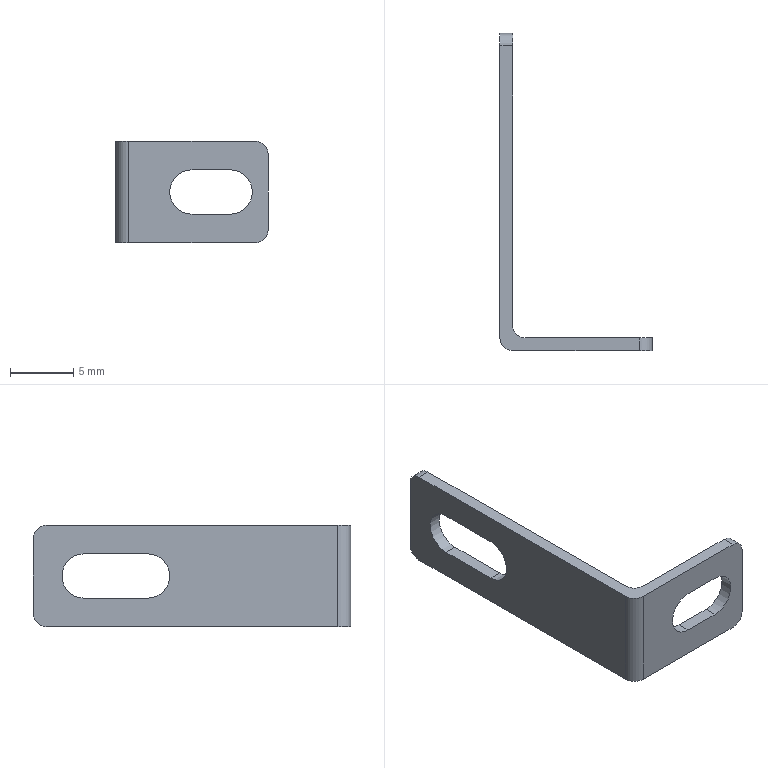Part | SolidWorks | features ICE 2, ExtruThin 1, Fillet 1 | 1 solid | 22 faces | box 12 x 25 x 8 mm | volume 239.899 mm3 | plane 12 | cylinder 10 | commonest cylinder face diameters 2 x6 3.5 x4
STEP:
#1=CARTESIAN_POINT('',(9.,0.,-1.75));
#2=VERTEX_POINT('',#1);
#3=CARTESIAN_POINT('',(6.,0.,-1.75));
#4=VERTEX_POINT('',#3);
#5=CARTESIAN_POINT('',(6.,0.,-1.75));
#6=DIRECTION('',(-1.,0.,0.));
#7=VECTOR('',#6,1000.);
#8=LINE('',#5,#7);
#9=EDGE_CURVE('',#2,#4,#8,.T.);
#10=ORIENTED_EDGE('',*,*,#9,.T.);
#11=CARTESIAN_POINT('',(6.,0.,1.75));
#12=VERTEX_POINT('',#11);
#13=CARTESIAN_POINT('',(6.,0.,0.));
#14=DIRECTION('',(0.,1.,0.));
#15=DIRECTION('',(0.,0.,1.));
#16=AXIS2_PLACEMENT_3D('',#13,#14,#15);
#17=CIRCLE('',#16,1.75);
#18=EDGE_CURVE('',#4,#12,#17,.T.);
#19=ORIENTED_EDGE('',*,*,#18,.T.);
#20=CARTESIAN_POINT('',(9.,0.,1.75));
#21=VERTEX_POINT('',#20);
#22=CARTESIAN_POINT('',(6.,0.,1.75));
#23=DIRECTION('',(1.,0.,0.));
#24=VECTOR('',#23,1000.);
#25=LINE('',#22,#24);
#26=EDGE_CURVE('',#12,#21,#25,.T.);
#27=ORIENTED_EDGE('',*,*,#26,.T.);
#28=CARTESIAN_POINT('',(9.,0.,0.));
#29=DIRECTION('',(0.,1.,0.));
#30=DIRECTION('',(0.,0.,1.));
#31=AXIS2_PLACEMENT_3D('',#28,#29,#30);
#32=CIRCLE('',#31,1.75);
#33=EDGE_CURVE('',#21,#2,#32,.T.);
#34=ORIENTED_EDGE('',*,*,#33,.T.);
#35=EDGE_LOOP('',(#10,#19,#27,#34));
#36=FACE_BOUND('',#35,.T.);
#37=CARTESIAN_POINT('',(1.,0.,-4.));
#38=VERTEX_POINT('',#37);
#39=CARTESIAN_POINT('',(11.,0.,-4.));
#40=VERTEX_POINT('',#39);
#41=CARTESIAN_POINT('',(0.,0.,-4.));
#42=DIRECTION('',(1.,0.,0.));
#43=VECTOR('',#42,1000.);
#44=LINE('',#41,#43);
#45=EDGE_CURVE('',#38,#40,#44,.T.);
#46=ORIENTED_EDGE('',*,*,#45,.T.);
#47=CARTESIAN_POINT('',(12.,0.,-3.));
#48=VERTEX_POINT('',#47);
#49=CARTESIAN_POINT('',(11.,0.,-3.));
#50=DIRECTION('',(0.,-1.,0.));
#51=DIRECTION('',(0.,0.,1.));
#52=AXIS2_PLACEMENT_3D('',#49,#50,#51);
#53=CIRCLE('',#52,1.);
#54=EDGE_CURVE('',#40,#48,#53,.T.);
#55=ORIENTED_EDGE('',*,*,#54,.T.);
#56=CARTESIAN_POINT('',(12.,0.,3.));
#57=VERTEX_POINT('',#56);
#58=CARTESIAN_POINT('',(12.,0.,4.));
#59=DIRECTION('',(0.,0.,-1.));
#60=VECTOR('',#59,1000.);
#61=LINE('',#58,#60);
#62=EDGE_CURVE('',#57,#48,#61,.T.);
#63=ORIENTED_EDGE('',*,*,#62,.F.);
#64=CARTESIAN_POINT('',(11.,0.,4.));
#65=VERTEX_POINT('',#64);
#66=CARTESIAN_POINT('',(11.,0.,3.));
#67=DIRECTION('',(0.,-1.,0.));
#68=DIRECTION('',(0.,0.,1.));
#69=AXIS2_PLACEMENT_3D('',#66,#67,#68);
#70=CIRCLE('',#69,1.);
#71=EDGE_CURVE('',#57,#65,#70,.T.);
#72=ORIENTED_EDGE('',*,*,#71,.T.);
#73=CARTESIAN_POINT('',(1.,0.,4.));
#74=VERTEX_POINT('',#73);
#75=CARTESIAN_POINT('',(0.,0.,4.));
#76=DIRECTION('',(1.,0.,0.));
#77=VECTOR('',#76,1000.);
#78=LINE('',#75,#77);
#79=EDGE_CURVE('',#74,#65,#78,.T.);
#80=ORIENTED_EDGE('',*,*,#79,.F.);
#81=CARTESIAN_POINT('',(1.,0.,4.));
#82=DIRECTION('',(0.,0.,-1.));
#83=VECTOR('',#82,1000.);
#84=LINE('',#81,#83);
#85=EDGE_CURVE('',#74,#38,#84,.T.);
#86=ORIENTED_EDGE('',*,*,#85,.T.);
#87=EDGE_LOOP('',(#46,#55,#63,#72,#80,#86));
#88=FACE_OUTER_BOUND('',#87,.T.);
#89=CARTESIAN_POINT('',(0.,0.,4.));
#90=DIRECTION('',(0.,1.,0.));
#91=DIRECTION('',(0.,0.,1.));
#92=AXIS2_PLACEMENT_3D('',#89,#90,#91);
#93=PLANE('',#92);
#94=ADVANCED_FACE('',(#36,#88),#93,.F.);
#95=ORIENTED_EDGE('',*,*,#62,.T.);
#96=CARTESIAN_POINT('',(12.,1.,-3.));
#97=VERTEX_POINT('',#96);
#98=CARTESIAN_POINT('',(12.,1.,-3.));
#99=DIRECTION('',(0.,1.,0.));
#100=VECTOR('',#99,1000.);
#101=LINE('',#98,#100);
#102=EDGE_CURVE('',#48,#97,#101,.T.);
#103=ORIENTED_EDGE('',*,*,#102,.T.);
#104=CARTESIAN_POINT('',(12.,1.,3.));
#105=VERTEX_POINT('',#104);
#106=CARTESIAN_POINT('',(12.,1.,4.));
#107=DIRECTION('',(0.,0.,-1.));
#108=VECTOR('',#107,1000.);
#109=LINE('',#106,#108);
#110=EDGE_CURVE('',#105,#97,#109,.T.);
#111=ORIENTED_EDGE('',*,*,#110,.F.);
#112=CARTESIAN_POINT('',(12.,0.,3.));
#113=DIRECTION('',(0.,-1.,0.));
#114=VECTOR('',#113,1000.);
#115=LINE('',#112,#114);
#116=EDGE_CURVE('',#105,#57,#115,.T.);
#117=ORIENTED_EDGE('',*,*,#116,.T.);
#118=EDGE_LOOP('',(#95,#103,#111,#117));
#119=FACE_OUTER_BOUND('',#118,.T.);
#120=CARTESIAN_POINT('',(12.,1.,4.));
#121=DIRECTION('',(1.,0.,0.));
#122=DIRECTION('',(0.,0.,-1.));
#123=AXIS2_PLACEMENT_3D('',#120,#121,#122);
#124=PLANE('',#123);
#125=ADVANCED_FACE('',(#119),#124,.T.);
#126=CARTESIAN_POINT('',(6.,1.,-1.75));
#127=VERTEX_POINT('',#126);
#128=CARTESIAN_POINT('',(6.,1.,1.75));
#129=VERTEX_POINT('',#128);
#130=CARTESIAN_POINT('',(6.,1.,0.));
#131=DIRECTION('',(0.,1.,0.));
#132=DIRECTION('',(0.,0.,1.));
#133=AXIS2_PLACEMENT_3D('',#130,#131,#132);
#134=CIRCLE('',#133,1.75);
#135=EDGE_CURVE('',#127,#129,#134,.T.);
#136=ORIENTED_EDGE('',*,*,#135,.F.);
#137=CARTESIAN_POINT('',(9.,1.,-1.75));
#138=VERTEX_POINT('',#137);
#139=CARTESIAN_POINT('',(6.,1.,-1.75));
#140=DIRECTION('',(-1.,0.,0.));
#141=VECTOR('',#140,1000.);
#142=LINE('',#139,#141);
#143=EDGE_CURVE('',#138,#127,#142,.T.);
#144=ORIENTED_EDGE('',*,*,#143,.F.);
#145=CARTESIAN_POINT('',(9.,1.,1.75));
#146=VERTEX_POINT('',#145);
#147=CARTESIAN_POINT('',(9.,1.,0.));
#148=DIRECTION('',(0.,1.,0.));
#149=DIRECTION('',(0.,0.,1.));
#150=AXIS2_PLACEMENT_3D('',#147,#148,#149);
#151=CIRCLE('',#150,1.75);
#152=EDGE_CURVE('',#146,#138,#151,.T.);
#153=ORIENTED_EDGE('',*,*,#152,.F.);
#154=CARTESIAN_POINT('',(6.,1.,1.75));
#155=DIRECTION('',(1.,0.,0.));
#156=VECTOR('',#155,1000.);
#157=LINE('',#154,#156);
#158=EDGE_CURVE('',#129,#146,#157,.T.);
#159=ORIENTED_EDGE('',*,*,#158,.F.);
#160=EDGE_LOOP('',(#136,#144,#153,#159));
#161=FACE_BOUND('',#160,.T.);
#162=ORIENTED_EDGE('',*,*,#110,.T.);
#163=CARTESIAN_POINT('',(11.,1.,-4.));
#164=VERTEX_POINT('',#163);
#165=CARTESIAN_POINT('',(11.,1.,-3.));
#166=DIRECTION('',(0.,1.,0.));
#167=DIRECTION('',(0.,0.,1.));
#168=AXIS2_PLACEMENT_3D('',#165,#166,#167);
#169=CIRCLE('',#168,1.);
#170=EDGE_CURVE('',#97,#164,#169,.T.);
#171=ORIENTED_EDGE('',*,*,#170,.T.);
#172=CARTESIAN_POINT('',(2.,1.,-4.));
#173=VERTEX_POINT('',#172);
#174=CARTESIAN_POINT('',(0.,1.,-4.));
#175=DIRECTION('',(1.,0.,0.));
#176=VECTOR('',#175,1000.);
#177=LINE('',#174,#176);
#178=EDGE_CURVE('',#173,#164,#177,.T.);
#179=ORIENTED_EDGE('',*,*,#178,.F.);
#180=CARTESIAN_POINT('',(2.,1.,4.));
#181=VERTEX_POINT('',#180);
#182=CARTESIAN_POINT('',(2.,1.,4.));
#183=DIRECTION('',(0.,0.,1.));
#184=VECTOR('',#183,1000.);
#185=LINE('',#182,#184);
#186=EDGE_CURVE('',#173,#181,#185,.T.);
#187=ORIENTED_EDGE('',*,*,#186,.T.);
#188=CARTESIAN_POINT('',(11.,1.,4.));
#189=VERTEX_POINT('',#188);
#190=CARTESIAN_POINT('',(0.,1.,4.));
#191=DIRECTION('',(1.,0.,0.));
#192=VECTOR('',#191,1000.);
#193=LINE('',#190,#192);
#194=EDGE_CURVE('',#181,#189,#193,.T.);
#195=ORIENTED_EDGE('',*,*,#194,.T.);
#196=CARTESIAN_POINT('',(11.,1.,3.));
#197=DIRECTION('',(0.,1.,0.));
#198=DIRECTION('',(0.,0.,1.));
#199=AXIS2_PLACEMENT_3D('',#196,#197,#198);
#200=CIRCLE('',#199,1.);
#201=EDGE_CURVE('',#189,#105,#200,.T.);
#202=ORIENTED_EDGE('',*,*,#201,.T.);
#203=EDGE_LOOP('',(#162,#171,#179,#187,#195,#202));
#204=FACE_OUTER_BOUND('',#203,.T.);
#205=CARTESIAN_POINT('',(0.,1.,4.));
#206=DIRECTION('',(0.,1.,0.));
#207=DIRECTION('',(0.,0.,1.));
#208=AXIS2_PLACEMENT_3D('',#205,#206,#207);
#209=PLANE('',#208);
#210=ADVANCED_FACE('',(#161,#204),#209,.T.);
#211=CARTESIAN_POINT('',(1.,16.,1.75));
#212=VERTEX_POINT('',#211);
#213=CARTESIAN_POINT('',(1.,16.,-1.75));
#214=VERTEX_POINT('',#213);
#215=CARTESIAN_POINT('',(1.,16.,0.));
#216=DIRECTION('',(1.,0.,0.));
#217=DIRECTION('',(0.,0.,-1.));
#218=AXIS2_PLACEMENT_3D('',#215,#216,#217);
#219=CIRCLE('',#218,1.75);
#220=EDGE_CURVE('',#212,#214,#219,.T.);
#221=ORIENTED_EDGE('',*,*,#220,.F.);
#222=CARTESIAN_POINT('',(1.,21.,1.75));
#223=VERTEX_POINT('',#222);
#224=CARTESIAN_POINT('',(1.,0.,1.75));
#225=DIRECTION('',(0.,-1.,0.));
#226=VECTOR('',#225,1000.);
#227=LINE('',#224,#226);
#228=EDGE_CURVE('',#223,#212,#227,.T.);
#229=ORIENTED_EDGE('',*,*,#228,.F.);
#230=CARTESIAN_POINT('',(1.,21.,-1.75));
#231=VERTEX_POINT('',#230);
#232=CARTESIAN_POINT('',(1.,21.,0.));
#233=DIRECTION('',(1.,0.,0.));
#234=DIRECTION('',(0.,0.,-1.));
#235=AXIS2_PLACEMENT_3D('',#232,#233,#234);
#236=CIRCLE('',#235,1.75);
#237=EDGE_CURVE('',#231,#223,#236,.T.);
#238=ORIENTED_EDGE('',*,*,#237,.F.);
#239=CARTESIAN_POINT('',(1.,0.,-1.75));
#240=DIRECTION('',(0.,1.,0.));
#241=VECTOR('',#240,1000.);
#242=LINE('',#239,#241);
#243=EDGE_CURVE('',#214,#231,#242,.T.);
#244=ORIENTED_EDGE('',*,*,#243,.F.);
#245=EDGE_LOOP('',(#221,#229,#238,#244));
#246=FACE_BOUND('',#245,.T.);
#247=CARTESIAN_POINT('',(1.,24.,-4.));
#248=VERTEX_POINT('',#247);
#249=CARTESIAN_POINT('',(1.,2.,-4.));
#250=VERTEX_POINT('',#249);
#251=CARTESIAN_POINT('',(1.,0.,-4.));
#252=DIRECTION('',(0.,-1.,0.));
#253=VECTOR('',#252,1000.);
#254=LINE('',#251,#253);
#255=EDGE_CURVE('',#248,#250,#254,.T.);
#256=ORIENTED_EDGE('',*,*,#255,.F.);
#257=CARTESIAN_POINT('',(1.,25.,-3.));
#258=VERTEX_POINT('',#257);
#259=CARTESIAN_POINT('',(1.,24.,-3.));
#260=DIRECTION('',(1.,0.,0.));
#261=DIRECTION('',(0.,0.,-1.));
#262=AXIS2_PLACEMENT_3D('',#259,#260,#261);
#263=CIRCLE('',#262,1.);
#264=EDGE_CURVE('',#248,#258,#263,.T.);
#265=ORIENTED_EDGE('',*,*,#264,.T.);
#266=CARTESIAN_POINT('',(1.,25.,3.));
#267=VERTEX_POINT('',#266);
#268=CARTESIAN_POINT('',(1.,25.,4.));
#269=DIRECTION('',(0.,0.,-1.));
#270=VECTOR('',#269,1000.);
#271=LINE('',#268,#270);
#272=EDGE_CURVE('',#267,#258,#271,.T.);
#273=ORIENTED_EDGE('',*,*,#272,.F.);
#274=CARTESIAN_POINT('',(1.,24.,4.));
#275=VERTEX_POINT('',#274);
#276=CARTESIAN_POINT('',(1.,24.,3.));
#277=DIRECTION('',(1.,0.,0.));
#278=DIRECTION('',(0.,0.,-1.));
#279=AXIS2_PLACEMENT_3D('',#276,#277,#278);
#280=CIRCLE('',#279,1.);
#281=EDGE_CURVE('',#267,#275,#280,.T.);
#282=ORIENTED_EDGE('',*,*,#281,.T.);
#283=CARTESIAN_POINT('',(1.,2.,4.));
#284=VERTEX_POINT('',#283);
#285=CARTESIAN_POINT('',(1.,0.,4.));
#286=DIRECTION('',(0.,-1.,0.));
#287=VECTOR('',#286,1000.);
#288=LINE('',#285,#287);
#289=EDGE_CURVE('',#275,#284,#288,.T.);
#290=ORIENTED_EDGE('',*,*,#289,.T.);
#291=CARTESIAN_POINT('',(1.,2.,-4.));
#292=DIRECTION('',(0.,0.,-1.));
#293=VECTOR('',#292,1000.);
#294=LINE('',#291,#293);
#295=EDGE_CURVE('',#284,#250,#294,.T.);
#296=ORIENTED_EDGE('',*,*,#295,.T.);
#297=EDGE_LOOP('',(#256,#265,#273,#282,#290,#296));
#298=FACE_OUTER_BOUND('',#297,.T.);
#299=CARTESIAN_POINT('',(1.,0.,4.));
#300=DIRECTION('',(1.,0.,0.));
#301=DIRECTION('',(0.,0.,-1.));
#302=AXIS2_PLACEMENT_3D('',#299,#300,#301);
#303=PLANE('',#302);
#304=ADVANCED_FACE('',(#246,#298),#303,.T.);
#305=ORIENTED_EDGE('',*,*,#272,.T.);
#306=CARTESIAN_POINT('',(0.,25.,-3.));
#307=VERTEX_POINT('',#306);
#308=CARTESIAN_POINT('',(0.,25.,-3.));
#309=DIRECTION('',(-1.,0.,0.));
#310=VECTOR('',#309,1000.);
#311=LINE('',#308,#310);
#312=EDGE_CURVE('',#258,#307,#311,.T.);
#313=ORIENTED_EDGE('',*,*,#312,.T.);
#314=CARTESIAN_POINT('',(0.,25.,3.));
#315=VERTEX_POINT('',#314);
#316=CARTESIAN_POINT('',(0.,25.,4.));
#317=DIRECTION('',(0.,0.,-1.));
#318=VECTOR('',#317,1000.);
#319=LINE('',#316,#318);
#320=EDGE_CURVE('',#315,#307,#319,.T.);
#321=ORIENTED_EDGE('',*,*,#320,.F.);
#322=CARTESIAN_POINT('',(1.,25.,3.));
#323=DIRECTION('',(1.,0.,0.));
#324=VECTOR('',#323,1000.);
#325=LINE('',#322,#324);
#326=EDGE_CURVE('',#315,#267,#325,.T.);
#327=ORIENTED_EDGE('',*,*,#326,.T.);
#328=EDGE_LOOP('',(#305,#313,#321,#327));
#329=FACE_OUTER_BOUND('',#328,.T.);
#330=CARTESIAN_POINT('',(0.,25.,4.));
#331=DIRECTION('',(0.,1.,0.));
#332=DIRECTION('',(0.,0.,1.));
#333=AXIS2_PLACEMENT_3D('',#330,#331,#332);
#334=PLANE('',#333);
#335=ADVANCED_FACE('',(#329),#334,.T.);
#336=CARTESIAN_POINT('',(0.,16.,1.75));
#337=VERTEX_POINT('',#336);
#338=CARTESIAN_POINT('',(0.,21.,1.75));
#339=VERTEX_POINT('',#338);
#340=CARTESIAN_POINT('',(0.,16.,1.75));
#341=DIRECTION('',(0.,1.,0.));
#342=VECTOR('',#341,1000.);
#343=LINE('',#340,#342);
#344=EDGE_CURVE('',#337,#339,#343,.T.);
#345=ORIENTED_EDGE('',*,*,#344,.F.);
#346=CARTESIAN_POINT('',(0.,16.,-1.75));
#347=VERTEX_POINT('',#346);
#348=CARTESIAN_POINT('',(0.,16.,0.));
#349=DIRECTION('',(-1.,0.,0.));
#350=DIRECTION('',(0.,0.,1.));
#351=AXIS2_PLACEMENT_3D('',#348,#349,#350);
#352=CIRCLE('',#351,1.75);
#353=EDGE_CURVE('',#347,#337,#352,.T.);
#354=ORIENTED_EDGE('',*,*,#353,.F.);
#355=CARTESIAN_POINT('',(0.,21.,-1.75));
#356=VERTEX_POINT('',#355);
#357=CARTESIAN_POINT('',(0.,16.,-1.75));
#358=DIRECTION('',(0.,-1.,0.));
#359=VECTOR('',#358,1000.);
#360=LINE('',#357,#359);
#361=EDGE_CURVE('',#356,#347,#360,.T.);
#362=ORIENTED_EDGE('',*,*,#361,.F.);
#363=CARTESIAN_POINT('',(0.,21.,0.));
#364=DIRECTION('',(-1.,0.,0.));
#365=DIRECTION('',(0.,0.,1.));
#366=AXIS2_PLACEMENT_3D('',#363,#364,#365);
#367=CIRCLE('',#366,1.75);
#368=EDGE_CURVE('',#339,#356,#367,.T.);
#369=ORIENTED_EDGE('',*,*,#368,.F.);
#370=EDGE_LOOP('',(#345,#354,#362,#369));
#371=FACE_BOUND('',#370,.T.);
#372=ORIENTED_EDGE('',*,*,#320,.T.);
#373=CARTESIAN_POINT('',(0.,24.,-4.));
#374=VERTEX_POINT('',#373);
#375=CARTESIAN_POINT('',(0.,24.,-3.));
#376=DIRECTION('',(-1.,0.,0.));
#377=DIRECTION('',(0.,0.,-1.));
#378=AXIS2_PLACEMENT_3D('',#375,#376,#377);
#379=CIRCLE('',#378,1.);
#380=EDGE_CURVE('',#307,#374,#379,.T.);
#381=ORIENTED_EDGE('',*,*,#380,.T.);
#382=CARTESIAN_POINT('',(0.,1.,-4.));
#383=VERTEX_POINT('',#382);
#384=CARTESIAN_POINT('',(0.,0.,-4.));
#385=DIRECTION('',(0.,-1.,0.));
#386=VECTOR('',#385,1000.);
#387=LINE('',#384,#386);
#388=EDGE_CURVE('',#374,#383,#387,.T.);
#389=ORIENTED_EDGE('',*,*,#388,.T.);
#390=CARTESIAN_POINT('',(0.,1.,4.));
#391=VERTEX_POINT('',#390);
#392=CARTESIAN_POINT('',(0.,1.,4.));
#393=DIRECTION('',(0.,0.,1.));
#394=VECTOR('',#393,1000.);
#395=LINE('',#392,#394);
#396=EDGE_CURVE('',#383,#391,#395,.T.);
#397=ORIENTED_EDGE('',*,*,#396,.T.);
#398=CARTESIAN_POINT('',(0.,24.,4.));
#399=VERTEX_POINT('',#398);
#400=CARTESIAN_POINT('',(0.,0.,4.));
#401=DIRECTION('',(0.,-1.,0.));
#402=VECTOR('',#401,1000.);
#403=LINE('',#400,#402);
#404=EDGE_CURVE('',#399,#391,#403,.T.);
#405=ORIENTED_EDGE('',*,*,#404,.F.);
#406=CARTESIAN_POINT('',(0.,24.,3.));
#407=DIRECTION('',(-1.,0.,0.));
#408=DIRECTION('',(0.,0.,-1.));
#409=AXIS2_PLACEMENT_3D('',#406,#407,#408);
#410=CIRCLE('',#409,1.);
#411=EDGE_CURVE('',#399,#315,#410,.T.);
#412=ORIENTED_EDGE('',*,*,#411,.T.);
#413=EDGE_LOOP('',(#372,#381,#389,#397,#405,#412));
#414=FACE_OUTER_BOUND('',#413,.T.);
#415=CARTESIAN_POINT('',(0.,0.,4.));
#416=DIRECTION('',(1.,0.,0.));
#417=DIRECTION('',(0.,0.,-1.));
#418=AXIS2_PLACEMENT_3D('',#415,#416,#417);
#419=PLANE('',#418);
#420=ADVANCED_FACE('',(#371,#414),#419,.F.);
#421=ORIENTED_EDGE('',*,*,#289,.F.);
#422=CARTESIAN_POINT('',(0.,24.,4.));
#423=DIRECTION('',(-1.,0.,0.));
#424=VECTOR('',#423,1000.);
#425=LINE('',#422,#424);
#426=EDGE_CURVE('',#275,#399,#425,.T.);
#427=ORIENTED_EDGE('',*,*,#426,.T.);
#428=ORIENTED_EDGE('',*,*,#404,.T.);
#429=CARTESIAN_POINT('',(1.,1.,4.));
#430=DIRECTION('',(0.,0.,1.));
#431=DIRECTION('',(-1.,0.,0.));
#432=AXIS2_PLACEMENT_3D('',#429,#430,#431);
#433=CIRCLE('',#432,1.);
#434=EDGE_CURVE('',#391,#74,#433,.T.);
#435=ORIENTED_EDGE('',*,*,#434,.T.);
#436=ORIENTED_EDGE('',*,*,#79,.T.);
#437=CARTESIAN_POINT('',(11.,1.,4.));
#438=DIRECTION('',(0.,1.,0.));
#439=VECTOR('',#438,1000.);
#440=LINE('',#437,#439);
#441=EDGE_CURVE('',#65,#189,#440,.T.);
#442=ORIENTED_EDGE('',*,*,#441,.T.);
#443=ORIENTED_EDGE('',*,*,#194,.F.);
#444=CARTESIAN_POINT('',(2.,2.,4.));
#445=DIRECTION('',(0.,0.,-1.));
#446=DIRECTION('',(-1.,0.,0.));
#447=AXIS2_PLACEMENT_3D('',#444,#445,#446);
#448=CIRCLE('',#447,1.);
#449=EDGE_CURVE('',#181,#284,#448,.T.);
#450=ORIENTED_EDGE('',*,*,#449,.T.);
#451=EDGE_LOOP('',(#421,#427,#428,#435,#436,#442,#443,#450));
#452=FACE_OUTER_BOUND('',#451,.T.);
#453=CARTESIAN_POINT('',(12.,0.,4.));
#454=DIRECTION('',(0.,0.,-1.));
#455=DIRECTION('',(-1.,0.,0.));
#456=AXIS2_PLACEMENT_3D('',#453,#454,#455);
#457=PLANE('',#456);
#458=ADVANCED_FACE('',(#452),#457,.F.);
#459=ORIENTED_EDGE('',*,*,#388,.F.);
#460=CARTESIAN_POINT('',(12.,24.,-4.));
#461=DIRECTION('',(1.,0.,0.));
#462=VECTOR('',#461,1000.);
#463=LINE('',#460,#462);
#464=EDGE_CURVE('',#374,#248,#463,.T.);
#465=ORIENTED_EDGE('',*,*,#464,.T.);
#466=ORIENTED_EDGE('',*,*,#255,.T.);
#467=CARTESIAN_POINT('',(2.,2.,-4.));
#468=DIRECTION('',(0.,0.,1.));
#469=DIRECTION('',(-1.,0.,0.));
#470=AXIS2_PLACEMENT_3D('',#467,#468,#469);
#471=CIRCLE('',#470,1.);
#472=EDGE_CURVE('',#250,#173,#471,.T.);
#473=ORIENTED_EDGE('',*,*,#472,.T.);
#474=ORIENTED_EDGE('',*,*,#178,.T.);
#475=CARTESIAN_POINT('',(11.,0.,-4.));
#476=DIRECTION('',(0.,-1.,0.));
#477=VECTOR('',#476,1000.);
#478=LINE('',#475,#477);
#479=EDGE_CURVE('',#164,#40,#478,.T.);
#480=ORIENTED_EDGE('',*,*,#479,.T.);
#481=ORIENTED_EDGE('',*,*,#45,.F.);
#482=CARTESIAN_POINT('',(1.,1.,-4.));
#483=DIRECTION('',(0.,0.,-1.));
#484=DIRECTION('',(-1.,0.,0.));
#485=AXIS2_PLACEMENT_3D('',#482,#483,#484);
#486=CIRCLE('',#485,1.);
#487=EDGE_CURVE('',#38,#383,#486,.T.);
#488=ORIENTED_EDGE('',*,*,#487,.T.);
#489=EDGE_LOOP('',(#459,#465,#466,#473,#474,#480,#481,#488));
#490=FACE_OUTER_BOUND('',#489,.T.);
#491=CARTESIAN_POINT('',(12.,0.,-4.));
#492=DIRECTION('',(0.,0.,-1.));
#493=DIRECTION('',(-1.,0.,0.));
#494=AXIS2_PLACEMENT_3D('',#491,#492,#493);
#495=PLANE('',#494);
#496=ADVANCED_FACE('',(#490),#495,.T.);
#497=ORIENTED_EDGE('',*,*,#135,.T.);
#498=CARTESIAN_POINT('',(6.,0.,1.75));
#499=DIRECTION('',(0.,1.,0.));
#500=VECTOR('',#499,1000.);
#501=LINE('',#498,#500);
#502=EDGE_CURVE('',#12,#129,#501,.T.);
#503=ORIENTED_EDGE('',*,*,#502,.F.);
#504=ORIENTED_EDGE('',*,*,#18,.F.);
#505=CARTESIAN_POINT('',(6.,0.,-1.75));
#506=DIRECTION('',(0.,1.,0.));
#507=VECTOR('',#506,1000.);
#508=LINE('',#505,#507);
#509=EDGE_CURVE('',#4,#127,#508,.T.);
#510=ORIENTED_EDGE('',*,*,#509,.T.);
#511=EDGE_LOOP('',(#497,#503,#504,#510));
#512=FACE_OUTER_BOUND('',#511,.T.);
#513=CARTESIAN_POINT('',(6.,0.,0.));
#514=DIRECTION('',(0.,1.,0.));
#515=DIRECTION('',(0.,0.,1.));
#516=AXIS2_PLACEMENT_3D('',#513,#514,#515);
#517=CYLINDRICAL_SURFACE('',#516,1.75);
#518=ADVANCED_FACE('',(#512),#517,.F.);
#519=ORIENTED_EDGE('',*,*,#143,.T.);
#520=ORIENTED_EDGE('',*,*,#509,.F.);
#521=ORIENTED_EDGE('',*,*,#9,.F.);
#522=CARTESIAN_POINT('',(9.,0.,-1.75));
#523=DIRECTION('',(0.,1.,0.));
#524=VECTOR('',#523,1000.);
#525=LINE('',#522,#524);
#526=EDGE_CURVE('',#2,#138,#525,.T.);
#527=ORIENTED_EDGE('',*,*,#526,.T.);
#528=EDGE_LOOP('',(#519,#520,#521,#527));
#529=FACE_OUTER_BOUND('',#528,.T.);
#530=CARTESIAN_POINT('',(6.,0.,-1.75));
#531=DIRECTION('',(0.,0.,-1.));
#532=DIRECTION('',(-1.,0.,0.));
#533=AXIS2_PLACEMENT_3D('',#530,#531,#532);
#534=PLANE('',#533);
#535=ADVANCED_FACE('',(#529),#534,.F.);
#536=ORIENTED_EDGE('',*,*,#152,.T.);
#537=ORIENTED_EDGE('',*,*,#526,.F.);
#538=ORIENTED_EDGE('',*,*,#33,.F.);
#539=CARTESIAN_POINT('',(9.,0.,1.75));
#540=DIRECTION('',(0.,1.,0.));
#541=VECTOR('',#540,1000.);
#542=LINE('',#539,#541);
#543=EDGE_CURVE('',#21,#146,#542,.T.);
#544=ORIENTED_EDGE('',*,*,#543,.T.);
#545=EDGE_LOOP('',(#536,#537,#538,#544));
#546=FACE_OUTER_BOUND('',#545,.T.);
#547=CARTESIAN_POINT('',(9.,0.,0.));
#548=DIRECTION('',(0.,1.,0.));
#549=DIRECTION('',(0.,0.,1.));
#550=AXIS2_PLACEMENT_3D('',#547,#548,#549);
#551=CYLINDRICAL_SURFACE('',#550,1.75);
#552=ADVANCED_FACE('',(#546),#551,.F.);
#553=ORIENTED_EDGE('',*,*,#158,.T.);
#554=ORIENTED_EDGE('',*,*,#543,.F.);
#555=ORIENTED_EDGE('',*,*,#26,.F.);
#556=ORIENTED_EDGE('',*,*,#502,.T.);
#557=EDGE_LOOP('',(#553,#554,#555,#556));
#558=FACE_OUTER_BOUND('',#557,.T.);
#559=CARTESIAN_POINT('',(6.,0.,1.75));
#560=DIRECTION('',(0.,0.,1.));
#561=DIRECTION('',(1.,0.,0.));
#562=AXIS2_PLACEMENT_3D('',#559,#560,#561);
#563=PLANE('',#562);
#564=ADVANCED_FACE('',(#558),#563,.F.);
#565=ORIENTED_EDGE('',*,*,#220,.T.);
#566=CARTESIAN_POINT('',(12.,16.,-1.75));
#567=DIRECTION('',(-1.,0.,0.));
#568=VECTOR('',#567,1000.);
#569=LINE('',#566,#568);
#570=EDGE_CURVE('',#214,#347,#569,.T.);
#571=ORIENTED_EDGE('',*,*,#570,.T.);
#572=ORIENTED_EDGE('',*,*,#353,.T.);
#573=CARTESIAN_POINT('',(12.,16.,1.75));
#574=DIRECTION('',(-1.,0.,0.));
#575=VECTOR('',#574,1000.);
#576=LINE('',#573,#575);
#577=EDGE_CURVE('',#212,#337,#576,.T.);
#578=ORIENTED_EDGE('',*,*,#577,.F.);
#579=EDGE_LOOP('',(#565,#571,#572,#578));
#580=FACE_OUTER_BOUND('',#579,.T.);
#581=CARTESIAN_POINT('',(12.,16.,0.));
#582=DIRECTION('',(-1.,0.,0.));
#583=DIRECTION('',(0.,0.,1.));
#584=AXIS2_PLACEMENT_3D('',#581,#582,#583);
#585=CYLINDRICAL_SURFACE('',#584,1.75);
#586=ADVANCED_FACE('',(#580),#585,.F.);
#587=ORIENTED_EDGE('',*,*,#243,.T.);
#588=CARTESIAN_POINT('',(12.,21.,-1.75));
#589=DIRECTION('',(-1.,0.,0.));
#590=VECTOR('',#589,1000.);
#591=LINE('',#588,#590);
#592=EDGE_CURVE('',#231,#356,#591,.T.);
#593=ORIENTED_EDGE('',*,*,#592,.T.);
#594=ORIENTED_EDGE('',*,*,#361,.T.);
#595=ORIENTED_EDGE('',*,*,#570,.F.);
#596=EDGE_LOOP('',(#587,#593,#594,#595));
#597=FACE_OUTER_BOUND('',#596,.T.);
#598=CARTESIAN_POINT('',(12.,16.,-1.75));
#599=DIRECTION('',(0.,0.,-1.));
#600=DIRECTION('',(-1.,0.,0.));
#601=AXIS2_PLACEMENT_3D('',#598,#599,#600);
#602=PLANE('',#601);
#603=ADVANCED_FACE('',(#597),#602,.F.);
#604=ORIENTED_EDGE('',*,*,#237,.T.);
#605=CARTESIAN_POINT('',(12.,21.,1.75));
#606=DIRECTION('',(-1.,0.,0.));
#607=VECTOR('',#606,1000.);
#608=LINE('',#605,#607);
#609=EDGE_CURVE('',#223,#339,#608,.T.);
#610=ORIENTED_EDGE('',*,*,#609,.T.);
#611=ORIENTED_EDGE('',*,*,#368,.T.);
#612=ORIENTED_EDGE('',*,*,#592,.F.);
#613=EDGE_LOOP('',(#604,#610,#611,#612));
#614=FACE_OUTER_BOUND('',#613,.T.);
#615=CARTESIAN_POINT('',(12.,21.,0.));
#616=DIRECTION('',(-1.,0.,0.));
#617=DIRECTION('',(0.,0.,1.));
#618=AXIS2_PLACEMENT_3D('',#615,#616,#617);
#619=CYLINDRICAL_SURFACE('',#618,1.75);
#620=ADVANCED_FACE('',(#614),#619,.F.);
#621=ORIENTED_EDGE('',*,*,#228,.T.);
#622=ORIENTED_EDGE('',*,*,#577,.T.);
#623=ORIENTED_EDGE('',*,*,#344,.T.);
#624=ORIENTED_EDGE('',*,*,#609,.F.);
#625=EDGE_LOOP('',(#621,#622,#623,#624));
#626=FACE_OUTER_BOUND('',#625,.T.);
#627=CARTESIAN_POINT('',(12.,16.,1.75));
#628=DIRECTION('',(0.,0.,1.));
#629=DIRECTION('',(1.,0.,0.));
#630=AXIS2_PLACEMENT_3D('',#627,#628,#629);
#631=PLANE('',#630);
#632=ADVANCED_FACE('',(#626),#631,.F.);
#633=ORIENTED_EDGE('',*,*,#380,.F.);
#634=ORIENTED_EDGE('',*,*,#312,.F.);
#635=ORIENTED_EDGE('',*,*,#264,.F.);
#636=ORIENTED_EDGE('',*,*,#464,.F.);
#637=EDGE_LOOP('',(#633,#634,#635,#636));
#638=FACE_OUTER_BOUND('',#637,.T.);
#639=CARTESIAN_POINT('',(12.,24.,-3.));
#640=DIRECTION('',(1.,0.,0.));
#641=DIRECTION('',(0.,0.,-1.));
#642=AXIS2_PLACEMENT_3D('',#639,#640,#641);
#643=CYLINDRICAL_SURFACE('',#642,1.);
#644=ADVANCED_FACE('',(#638),#643,.T.);
#645=ORIENTED_EDGE('',*,*,#411,.F.);
#646=ORIENTED_EDGE('',*,*,#426,.F.);
#647=ORIENTED_EDGE('',*,*,#281,.F.);
#648=ORIENTED_EDGE('',*,*,#326,.F.);
#649=EDGE_LOOP('',(#645,#646,#647,#648));
#650=FACE_OUTER_BOUND('',#649,.T.);
#651=CARTESIAN_POINT('',(0.,24.,3.));
#652=DIRECTION('',(-1.,0.,0.));
#653=DIRECTION('',(0.,0.,1.));
#654=AXIS2_PLACEMENT_3D('',#651,#652,#653);
#655=CYLINDRICAL_SURFACE('',#654,1.);
#656=ADVANCED_FACE('',(#650),#655,.T.);
#657=ORIENTED_EDGE('',*,*,#170,.F.);
#658=ORIENTED_EDGE('',*,*,#102,.F.);
#659=ORIENTED_EDGE('',*,*,#54,.F.);
#660=ORIENTED_EDGE('',*,*,#479,.F.);
#661=EDGE_LOOP('',(#657,#658,#659,#660));
#662=FACE_OUTER_BOUND('',#661,.T.);
#663=CARTESIAN_POINT('',(11.,0.,-3.));
#664=DIRECTION('',(0.,-1.,0.));
#665=DIRECTION('',(0.,0.,-1.));
#666=AXIS2_PLACEMENT_3D('',#663,#664,#665);
#667=CYLINDRICAL_SURFACE('',#666,1.);
#668=ADVANCED_FACE('',(#662),#667,.T.);
#669=ORIENTED_EDGE('',*,*,#201,.F.);
#670=ORIENTED_EDGE('',*,*,#441,.F.);
#671=ORIENTED_EDGE('',*,*,#71,.F.);
#672=ORIENTED_EDGE('',*,*,#116,.F.);
#673=EDGE_LOOP('',(#669,#670,#671,#672));
#674=FACE_OUTER_BOUND('',#673,.T.);
#675=CARTESIAN_POINT('',(11.,1.,3.));
#676=DIRECTION('',(0.,1.,0.));
#677=DIRECTION('',(0.,0.,1.));
#678=AXIS2_PLACEMENT_3D('',#675,#676,#677);
#679=CYLINDRICAL_SURFACE('',#678,1.);
#680=ADVANCED_FACE('',(#674),#679,.T.);
#681=ORIENTED_EDGE('',*,*,#434,.F.);
#682=ORIENTED_EDGE('',*,*,#396,.F.);
#683=ORIENTED_EDGE('',*,*,#487,.F.);
#684=ORIENTED_EDGE('',*,*,#85,.F.);
#685=EDGE_LOOP('',(#681,#682,#683,#684));
#686=FACE_OUTER_BOUND('',#685,.T.);
#687=CARTESIAN_POINT('',(1.,1.,4.));
#688=DIRECTION('',(0.,0.,-1.));
#689=DIRECTION('',(-1.,0.,0.));
#690=AXIS2_PLACEMENT_3D('',#687,#688,#689);
#691=CYLINDRICAL_SURFACE('',#690,1.);
#692=ADVANCED_FACE('',(#686),#691,.T.);
#693=ORIENTED_EDGE('',*,*,#449,.F.);
#694=ORIENTED_EDGE('',*,*,#186,.F.);
#695=ORIENTED_EDGE('',*,*,#472,.F.);
#696=ORIENTED_EDGE('',*,*,#295,.F.);
#697=EDGE_LOOP('',(#693,#694,#695,#696));
#698=FACE_OUTER_BOUND('',#697,.T.);
#699=CARTESIAN_POINT('',(2.,2.,4.));
#700=DIRECTION('',(0.,0.,1.));
#701=DIRECTION('',(1.,0.,0.));
#702=AXIS2_PLACEMENT_3D('',#699,#700,#701);
#703=CYLINDRICAL_SURFACE('',#702,1.);
#704=ADVANCED_FACE('',(#698),#703,.F.);
#705=CLOSED_SHELL('',(#94,#125,#210,#304,#335,#420,#458,#496,#518,#535,#552,#564,#586,#603,#620,#632,#644,#656,#668,#680,#692,#704));
#706=MANIFOLD_SOLID_BREP('',#705);
#707=CARTESIAN_POINT('',(0.,0.,0.));
#708=DIRECTION('',(0.,0.,1.));
#709=DIRECTION('',(1.,0.,0.));
#710=AXIS2_PLACEMENT_3D('',#707,#708,#709);
#711=(LENGTH_UNIT()NAMED_UNIT(*)SI_UNIT(.MILLI.,.METRE.));
#712=UNCERTAINTY_MEASURE_WITH_UNIT(LENGTH_MEASURE(0.00001),#711,'','');
#713=(NAMED_UNIT(*)PLANE_ANGLE_UNIT()SI_UNIT($,.RADIAN.));
#714=(NAMED_UNIT(*)SI_UNIT($,.STERADIAN.)SOLID_ANGLE_UNIT());
#715=(GEOMETRIC_REPRESENTATION_CONTEXT(3)GLOBAL_UNCERTAINTY_ASSIGNED_CONTEXT((#712))GLOBAL_UNIT_ASSIGNED_CONTEXT((#711,#713,#714))REPRESENTATION_CONTEXT('',''));
#716=ADVANCED_BREP_SHAPE_REPRESENTATION('',(#706,#710),#715);